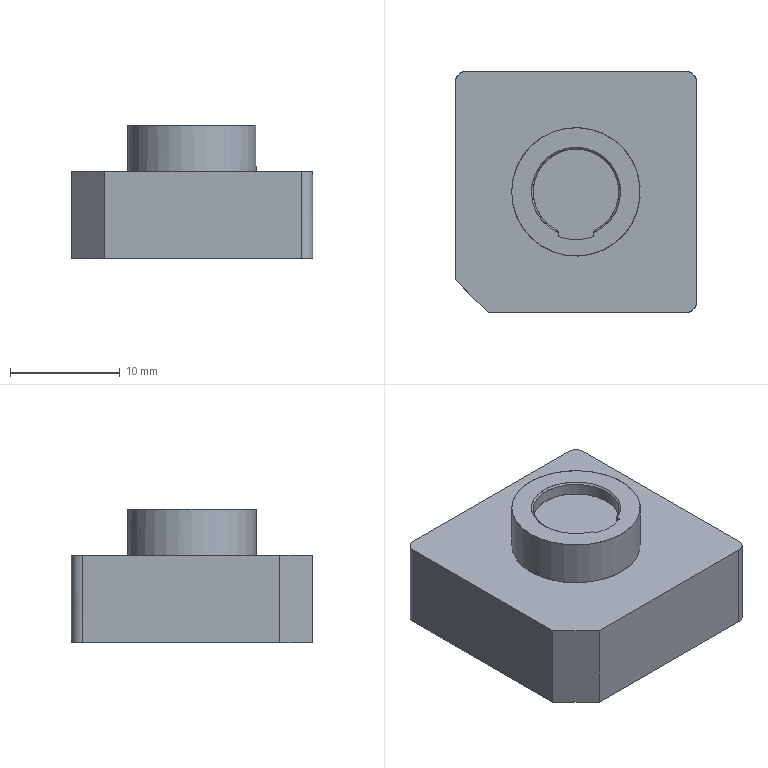CAM job | PowerMill | 3-axis milling, other | part box 22 x 22 x 12.219 mm
Tools:
number,name,type,diameter,tip_radius,length,cutting_length,overhang,flutes,holder,toolpaths_using
1,D10C,end_mill,10.0,0.0,60.0,,30.0,1,D42L35,1
1,D10C_1_1,end_mill,10.0,0.0,60.0,,12.68,1,D42L35,3
15,D3C_1_1,end_mill,3.0,0.0,30.0,,4.4,1,D42L35,1
3,D10_1_1,end_mill,10.0,0.0,60.0,,12.36,1,D42L35,4
12,D2_1_1,end_mill,2.0,0.0,4.36,,4.36,1,D42L35,2
17,D0.8_1_1,end_mill,0.8,0.0,1.48,,1.48,1,D42L35,1
13,Text_D4_1_1,taper_spherical,4.0,0.3,60.0,,4.48,1,D42L35,1
Operations:
program,toolpath,strategy,tool,tool_number,tool_diameter,tip_radius,flutes,spindle_rpm,feed_cut,surface_speed_m_min_computed,feed_per_tooth_computed,tolerance,thickness,stepover,stepdown,cut_length,cut_time_min,total_time_min,workplane
18-0710-1-F,精公开粗01-扫面平行-D10C,raster_area_clear,D10C_1_1,1,10.0,0.0,1.0,8000.0,10000.0,251.33,1.25,0.03,0.28,6.0,1.0,192.92,0.019,0.0239,
18-0710-1-F,精公开粗01-外形偏置-D10C,offset_area_clear,D10C_1_1,1,10.0,0.0,1.0,8000.0,10000.0,251.33,1.25,0.03,0.28,6.0,1.0,2021.961,0.202,0.2314,
18-0710-1-F,精公开粗01-基准台等高-D10C,constantz,D10C_1_1,1,10.0,0.0,1.0,8000.0,10000.0,251.33,1.25,0.03,0.07,5.0,0.4,2568.985,0.257,0.2651,
18-0710-1-F,精公再粗02-外形偏置-D3C,offset_area_clear,D3C_1_1,15,3.0,0.0,1.0,18000.0,5000.0,169.65,0.2778,0.03,0.0,2.0,1.0,1710.638,0.342,0.4029,
18-0710-1-F,精公基准台01-平坦面平行-D10,raster_area_clear,D10_1_1,3,10.0,0.0,1.0,8500.0,600.0,267.04,0.0706,0.005,0.38,5.0,1.0,95.295,0.159,0.1749,
18-0710-1-F,精公基准台01-基准面偏置-D10,offset_area_clear,D10_1_1,3,10.0,0.0,1.0,8500.0,600.0,267.04,0.0706,0.005,0.38,5.0,1.0,81.465,0.136,0.153,
18-0710-1-F,精公基准台01-外形侧光-D10,profile_area_clear,D10_1_1,3,10.0,0.0,1.0,8500.0,600.0,267.04,0.0706,0.005,-0.07,0.08,1.0,136.066,0.227,0.2456,
18-0710-1-F,精公基准台01-基准台侧光-D10,profile_area_clear,D10_1_1,3,10.0,0.0,1.0,8500.0,600.0,267.04,0.0706,0.005,0.0,0.08,1.0,233.232,0.389,0.4514,
18-0710-1-F,精公精光01-等高-D2,constantz,D2_1_1,12,2.0,0.0,1.0,18000.0,1500.0,113.1,0.0833,0.005,-0.075,5.0,0.03,6738.004,4.492,4.5,
18-0710-1-F,精公精光01-平坦面偏置-D2,offset_area_clear,D2_1_1,12,2.0,0.0,1.0,18000.0,600.0,113.1,0.0333,0.005,0.375,1.0,1.0,152.01,0.253,0.2923,
18-0710-1-F,精公精光02-等高-D0.8,constantz,D0.8_1_1,17,0.8,0.0,1.0,20000.0,600.0,50.27,0.03,0.005,-0.075,5.0,0.02,189.443,0.316,0.4117,
18-0710-1-F,精公刻字01-刻字-Text_D4,pattern,Text_D4_1_1,13,4.0,0.3,1.0,15000.0,1000.0,188.5,0.0667,0.005,0.0,5.0,1.0,32.413,0.032,0.0488,
,精公开粗01-外形偏置-D10C_Reference,offset_area_clear,D10C,1,10.0,0.0,1.0,8000.0,10000.0,251.33,1.25,0.03,0.28,6.0,1.0,5146.81,0.515,0.5851,